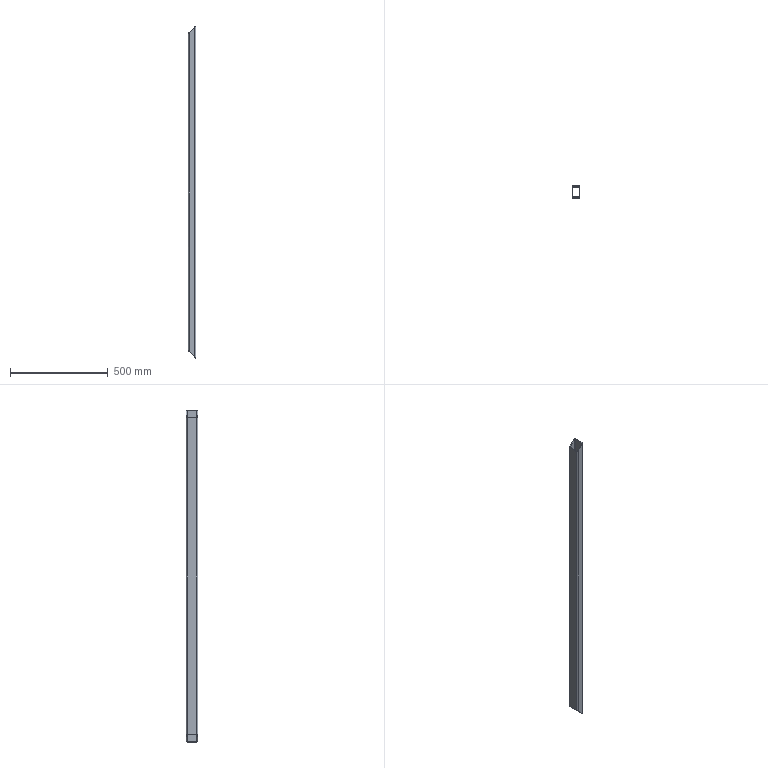Part | STEP file | Profile 40601700 | 1 solid | 18 faces | box 40 x 60 x 1700 mm | volume 950632 mm3 | plane 10 | cylinder 8 | commonest cylinder face diameters 6.4 x4 12.8 x4
STEP:
#1=CARTESIAN_POINT('',(40.,6.4,1100.));
#2=VERTEX_POINT('',#1);
#3=CARTESIAN_POINT('',(40.,53.6,1100.));
#4=VERTEX_POINT('',#3);
#5=CARTESIAN_POINT('',(40.,53.6,1100.));
#6=DIRECTION('',(0.,1.,0.));
#7=VECTOR('',#6,1000.);
#8=LINE('',#5,#7);
#9=EDGE_CURVE('',#2,#4,#8,.T.);
#10=ORIENTED_EDGE('',*,*,#9,.F.);
#11=CARTESIAN_POINT('',(40.,6.4,-600.));
#12=VERTEX_POINT('',#11);
#13=CARTESIAN_POINT('',(40.,6.4,600.));
#14=DIRECTION('',(0.,0.,1.));
#15=VECTOR('',#14,1000.);
#16=LINE('',#13,#15);
#17=EDGE_CURVE('',#12,#2,#16,.T.);
#18=ORIENTED_EDGE('',*,*,#17,.F.);
#19=CARTESIAN_POINT('',(40.,53.6,-600.));
#20=VERTEX_POINT('',#19);
#21=CARTESIAN_POINT('',(40.,53.6,-600.));
#22=DIRECTION('',(0.,-1.,0.));
#23=VECTOR('',#22,1000.);
#24=LINE('',#21,#23);
#25=EDGE_CURVE('',#20,#12,#24,.T.);
#26=ORIENTED_EDGE('',*,*,#25,.F.);
#27=CARTESIAN_POINT('',(40.,53.6,600.));
#28=DIRECTION('',(0.,0.,-1.));
#29=VECTOR('',#28,1000.);
#30=LINE('',#27,#29);
#31=EDGE_CURVE('',#4,#20,#30,.T.);
#32=ORIENTED_EDGE('',*,*,#31,.F.);
#33=EDGE_LOOP('',(#10,#18,#26,#32));
#34=FACE_OUTER_BOUND('',#33,.T.);
#35=CARTESIAN_POINT('',(40.,53.6,600.));
#36=DIRECTION('',(-1.,0.,0.));
#37=DIRECTION('',(0.,0.,1.));
#38=AXIS2_PLACEMENT_3D('',#35,#36,#37);
#39=PLANE('',#38);
#40=ADVANCED_FACE('',(#34),#39,.F.);
#41=CARTESIAN_POINT('',(33.6,60.,-593.6));
#42=VERTEX_POINT('',#41);
#43=CARTESIAN_POINT('',(40.,53.6,-600.));
#44=CARTESIAN_POINT('',(40.,57.349,-600.));
#45=CARTESIAN_POINT('',(37.349,60.,-597.349));
#46=CARTESIAN_POINT('',(33.6,60.,-593.6));
#47=(BOUNDED_CURVE()B_SPLINE_CURVE(3,(#43,#44,#45,#46),.UNSPECIFIED.,.F.,.F.)B_SPLINE_CURVE_WITH_KNOTS((4,4),(0.,1.571),.UNSPECIFIED.)CURVE()GEOMETRIC_REPRESENTATION_ITEM()RATIONAL_B_SPLINE_CURVE((1.,0.8047,0.8047,1.))REPRESENTATION_ITEM(''));
#48=EDGE_CURVE('',#20,#42,#47,.T.);
#49=ORIENTED_EDGE('',*,*,#48,.T.);
#50=CARTESIAN_POINT('',(33.6,60.,1093.6));
#51=VERTEX_POINT('',#50);
#52=CARTESIAN_POINT('',(33.6,60.,600.));
#53=DIRECTION('',(0.,0.,1.));
#54=VECTOR('',#53,1000.);
#55=LINE('',#52,#54);
#56=EDGE_CURVE('',#42,#51,#55,.T.);
#57=ORIENTED_EDGE('',*,*,#56,.T.);
#58=CARTESIAN_POINT('',(33.6,60.,1093.6));
#59=CARTESIAN_POINT('',(37.349,60.,1097.349));
#60=CARTESIAN_POINT('',(40.,57.349,1100.));
#61=CARTESIAN_POINT('',(40.,53.6,1100.));
#62=(BOUNDED_CURVE()B_SPLINE_CURVE(3,(#58,#59,#60,#61),.UNSPECIFIED.,.F.,.F.)B_SPLINE_CURVE_WITH_KNOTS((4,4),(1.571,3.142),.UNSPECIFIED.)CURVE()GEOMETRIC_REPRESENTATION_ITEM()RATIONAL_B_SPLINE_CURVE((1.,0.8047,0.8047,1.))REPRESENTATION_ITEM(''));
#63=EDGE_CURVE('',#51,#4,#62,.T.);
#64=ORIENTED_EDGE('',*,*,#63,.T.);
#65=ORIENTED_EDGE('',*,*,#31,.T.);
#66=EDGE_LOOP('',(#49,#57,#64,#65));
#67=FACE_OUTER_BOUND('',#66,.T.);
#68=CARTESIAN_POINT('',(33.6,53.6,600.));
#69=DIRECTION('',(0.,0.,-1.));
#70=DIRECTION('',(-1.,0.,0.));
#71=AXIS2_PLACEMENT_3D('',#68,#69,#70);
#72=CYLINDRICAL_SURFACE('',#71,6.4);
#73=ADVANCED_FACE('',(#67),#72,.T.);
#74=CARTESIAN_POINT('',(36.8,53.6,1096.8));
#75=VERTEX_POINT('',#74);
#76=CARTESIAN_POINT('',(33.6,56.8,1093.6));
#77=VERTEX_POINT('',#76);
#78=CARTESIAN_POINT('',(36.8,53.6,1096.8));
#79=CARTESIAN_POINT('',(36.8,55.475,1096.8));
#80=CARTESIAN_POINT('',(35.475,56.8,1095.475));
#81=CARTESIAN_POINT('',(33.6,56.8,1093.6));
#82=(BOUNDED_CURVE()B_SPLINE_CURVE(3,(#78,#79,#80,#81),.UNSPECIFIED.,.F.,.F.)B_SPLINE_CURVE_WITH_KNOTS((4,4),(3.142,4.712),.UNSPECIFIED.)CURVE()GEOMETRIC_REPRESENTATION_ITEM()RATIONAL_B_SPLINE_CURVE((1.,0.8047,0.8047,1.))REPRESENTATION_ITEM(''));
#83=EDGE_CURVE('',#75,#77,#82,.T.);
#84=ORIENTED_EDGE('',*,*,#83,.F.);
#85=CARTESIAN_POINT('',(36.8,6.4,1096.8));
#86=VERTEX_POINT('',#85);
#87=CARTESIAN_POINT('',(36.8,-440.,1096.8));
#88=DIRECTION('',(0.,1.,0.));
#89=VECTOR('',#88,1000.);
#90=LINE('',#87,#89);
#91=EDGE_CURVE('',#86,#75,#90,.T.);
#92=ORIENTED_EDGE('',*,*,#91,.F.);
#93=CARTESIAN_POINT('',(33.6,3.2,1093.6));
#94=VERTEX_POINT('',#93);
#95=CARTESIAN_POINT('',(33.6,3.2,1093.6));
#96=CARTESIAN_POINT('',(35.475,3.2,1095.475));
#97=CARTESIAN_POINT('',(36.8,4.525,1096.8));
#98=CARTESIAN_POINT('',(36.8,6.4,1096.8));
#99=(BOUNDED_CURVE()B_SPLINE_CURVE(3,(#95,#96,#97,#98),.UNSPECIFIED.,.F.,.T.)B_SPLINE_CURVE_WITH_KNOTS((4,4),(1.571,3.142),.UNSPECIFIED.)CURVE()GEOMETRIC_REPRESENTATION_ITEM()RATIONAL_B_SPLINE_CURVE((1.,0.8047,0.8047,1.))REPRESENTATION_ITEM(''));
#100=EDGE_CURVE('',#94,#86,#99,.T.);
#101=ORIENTED_EDGE('',*,*,#100,.F.);
#102=CARTESIAN_POINT('',(6.4,3.2,1066.4));
#103=VERTEX_POINT('',#102);
#104=CARTESIAN_POINT('',(0.,3.2,1060.));
#105=DIRECTION('',(0.7071,0.,0.7071));
#106=VECTOR('',#105,1000.);
#107=LINE('',#104,#106);
#108=EDGE_CURVE('',#103,#94,#107,.T.);
#109=ORIENTED_EDGE('',*,*,#108,.F.);
#110=CARTESIAN_POINT('',(3.2,6.4,1063.2));
#111=VERTEX_POINT('',#110);
#112=CARTESIAN_POINT('',(3.2,6.4,1063.2));
#113=CARTESIAN_POINT('',(3.2,4.525,1063.2));
#114=CARTESIAN_POINT('',(4.525,3.2,1064.525));
#115=CARTESIAN_POINT('',(6.4,3.2,1066.4));
#116=(BOUNDED_CURVE()B_SPLINE_CURVE(3,(#112,#113,#114,#115),.UNSPECIFIED.,.F.,.F.)B_SPLINE_CURVE_WITH_KNOTS((4,4),(0.,1.571),.UNSPECIFIED.)CURVE()GEOMETRIC_REPRESENTATION_ITEM()RATIONAL_B_SPLINE_CURVE((1.,0.8047,0.8047,1.))REPRESENTATION_ITEM(''));
#117=EDGE_CURVE('',#111,#103,#116,.T.);
#118=ORIENTED_EDGE('',*,*,#117,.F.);
#119=CARTESIAN_POINT('',(3.2,53.6,1063.2));
#120=VERTEX_POINT('',#119);
#121=CARTESIAN_POINT('',(3.2,-440.,1063.2));
#122=DIRECTION('',(0.,-1.,0.));
#123=VECTOR('',#122,1000.);
#124=LINE('',#121,#123);
#125=EDGE_CURVE('',#120,#111,#124,.T.);
#126=ORIENTED_EDGE('',*,*,#125,.F.);
#127=CARTESIAN_POINT('',(6.4,56.8,1066.4));
#128=VERTEX_POINT('',#127);
#129=CARTESIAN_POINT('',(6.4,56.8,1066.4));
#130=CARTESIAN_POINT('',(4.525,56.8,1064.525));
#131=CARTESIAN_POINT('',(3.2,55.475,1063.2));
#132=CARTESIAN_POINT('',(3.2,53.6,1063.2));
#133=(BOUNDED_CURVE()B_SPLINE_CURVE(3,(#129,#130,#131,#132),.UNSPECIFIED.,.F.,.F.)B_SPLINE_CURVE_WITH_KNOTS((4,4),(4.712,6.283),.UNSPECIFIED.)CURVE()GEOMETRIC_REPRESENTATION_ITEM()RATIONAL_B_SPLINE_CURVE((1.,0.8047,0.8047,1.))REPRESENTATION_ITEM(''));
#134=EDGE_CURVE('',#128,#120,#133,.T.);
#135=ORIENTED_EDGE('',*,*,#134,.F.);
#136=CARTESIAN_POINT('',(0.,56.8,1060.));
#137=DIRECTION('',(-0.7071,0.,-0.7071));
#138=VECTOR('',#137,1000.);
#139=LINE('',#136,#138);
#140=EDGE_CURVE('',#77,#128,#139,.T.);
#141=ORIENTED_EDGE('',*,*,#140,.F.);
#142=EDGE_LOOP('',(#84,#92,#101,#109,#118,#126,#135,#141));
#143=FACE_BOUND('',#142,.T.);
#144=CARTESIAN_POINT('',(6.4,60.,1066.4));
#145=VERTEX_POINT('',#144);
#146=CARTESIAN_POINT('',(0.,60.,1060.));
#147=DIRECTION('',(0.7071,0.,0.7071));
#148=VECTOR('',#147,1000.);
#149=LINE('',#146,#148);
#150=EDGE_CURVE('',#145,#51,#149,.T.);
#151=ORIENTED_EDGE('',*,*,#150,.F.);
#152=CARTESIAN_POINT('',(0.,53.6,1060.));
#153=VERTEX_POINT('',#152);
#154=CARTESIAN_POINT('',(0.,53.6,1060.));
#155=CARTESIAN_POINT('',(0.,57.349,1060.));
#156=CARTESIAN_POINT('',(2.651,60.,1062.651));
#157=CARTESIAN_POINT('',(6.4,60.,1066.4));
#158=(BOUNDED_CURVE()B_SPLINE_CURVE(3,(#154,#155,#156,#157),.UNSPECIFIED.,.F.,.T.)B_SPLINE_CURVE_WITH_KNOTS((4,4),(0.,1.571),.UNSPECIFIED.)CURVE()GEOMETRIC_REPRESENTATION_ITEM()RATIONAL_B_SPLINE_CURVE((1.,0.8047,0.8047,1.))REPRESENTATION_ITEM(''));
#159=EDGE_CURVE('',#153,#145,#158,.T.);
#160=ORIENTED_EDGE('',*,*,#159,.F.);
#161=CARTESIAN_POINT('',(0.,6.4,1060.));
#162=VERTEX_POINT('',#161);
#163=CARTESIAN_POINT('',(0.,-440.,1060.));
#164=DIRECTION('',(0.,1.,0.));
#165=VECTOR('',#164,1000.);
#166=LINE('',#163,#165);
#167=EDGE_CURVE('',#162,#153,#166,.T.);
#168=ORIENTED_EDGE('',*,*,#167,.F.);
#169=CARTESIAN_POINT('',(6.4,0.,1066.4));
#170=VERTEX_POINT('',#169);
#171=CARTESIAN_POINT('',(6.4,0.,1066.4));
#172=CARTESIAN_POINT('',(2.651,0.,1062.651));
#173=CARTESIAN_POINT('',(0.,2.651,1060.));
#174=CARTESIAN_POINT('',(0.,6.4,1060.));
#175=(BOUNDED_CURVE()B_SPLINE_CURVE(3,(#171,#172,#173,#174),.UNSPECIFIED.,.F.,.F.)B_SPLINE_CURVE_WITH_KNOTS((4,4),(4.712,6.283),.UNSPECIFIED.)CURVE()GEOMETRIC_REPRESENTATION_ITEM()RATIONAL_B_SPLINE_CURVE((1.,0.8047,0.8047,1.))REPRESENTATION_ITEM(''));
#176=EDGE_CURVE('',#170,#162,#175,.T.);
#177=ORIENTED_EDGE('',*,*,#176,.F.);
#178=CARTESIAN_POINT('',(33.6,0.,1093.6));
#179=VERTEX_POINT('',#178);
#180=CARTESIAN_POINT('',(0.,0.,1060.));
#181=DIRECTION('',(-0.7071,0.,-0.7071));
#182=VECTOR('',#181,1000.);
#183=LINE('',#180,#182);
#184=EDGE_CURVE('',#179,#170,#183,.T.);
#185=ORIENTED_EDGE('',*,*,#184,.F.);
#186=CARTESIAN_POINT('',(40.,6.4,1100.));
#187=CARTESIAN_POINT('',(40.,2.651,1100.));
#188=CARTESIAN_POINT('',(37.349,0.,1097.349));
#189=CARTESIAN_POINT('',(33.6,0.,1093.6));
#190=(BOUNDED_CURVE()B_SPLINE_CURVE(3,(#186,#187,#188,#189),.UNSPECIFIED.,.F.,.F.)B_SPLINE_CURVE_WITH_KNOTS((4,4),(3.142,4.712),.UNSPECIFIED.)CURVE()GEOMETRIC_REPRESENTATION_ITEM()RATIONAL_B_SPLINE_CURVE((1.,0.8047,0.8047,1.))REPRESENTATION_ITEM(''));
#191=EDGE_CURVE('',#2,#179,#190,.T.);
#192=ORIENTED_EDGE('',*,*,#191,.F.);
#193=ORIENTED_EDGE('',*,*,#9,.T.);
#194=ORIENTED_EDGE('',*,*,#63,.F.);
#195=EDGE_LOOP('',(#151,#160,#168,#177,#185,#192,#193,#194));
#196=FACE_OUTER_BOUND('',#195,.T.);
#197=CARTESIAN_POINT('',(0.,-440.,1060.));
#198=DIRECTION('',(0.7071,0.,-0.7071));
#199=DIRECTION('',(-0.7071,0.,-0.7071));
#200=AXIS2_PLACEMENT_3D('',#197,#198,#199);
#201=PLANE('',#200);
#202=ADVANCED_FACE('',(#143,#196),#201,.F.);
#203=CARTESIAN_POINT('',(33.6,0.,-593.6));
#204=VERTEX_POINT('',#203);
#205=CARTESIAN_POINT('',(33.6,0.,-593.6));
#206=CARTESIAN_POINT('',(37.349,0.,-597.349));
#207=CARTESIAN_POINT('',(40.,2.651,-600.));
#208=CARTESIAN_POINT('',(40.,6.4,-600.));
#209=(BOUNDED_CURVE()B_SPLINE_CURVE(3,(#205,#206,#207,#208),.UNSPECIFIED.,.F.,.F.)B_SPLINE_CURVE_WITH_KNOTS((4,4),(4.712,6.283),.UNSPECIFIED.)CURVE()GEOMETRIC_REPRESENTATION_ITEM()RATIONAL_B_SPLINE_CURVE((1.,0.8047,0.8047,1.))REPRESENTATION_ITEM(''));
#210=EDGE_CURVE('',#204,#12,#209,.T.);
#211=ORIENTED_EDGE('',*,*,#210,.T.);
#212=ORIENTED_EDGE('',*,*,#17,.T.);
#213=ORIENTED_EDGE('',*,*,#191,.T.);
#214=CARTESIAN_POINT('',(33.6,0.,600.));
#215=DIRECTION('',(0.,0.,-1.));
#216=VECTOR('',#215,1000.);
#217=LINE('',#214,#216);
#218=EDGE_CURVE('',#179,#204,#217,.T.);
#219=ORIENTED_EDGE('',*,*,#218,.T.);
#220=EDGE_LOOP('',(#211,#212,#213,#219));
#221=FACE_OUTER_BOUND('',#220,.T.);
#222=CARTESIAN_POINT('',(33.6,6.4,600.));
#223=DIRECTION('',(0.,0.,-1.));
#224=DIRECTION('',(-1.,0.,0.));
#225=AXIS2_PLACEMENT_3D('',#222,#223,#224);
#226=CYLINDRICAL_SURFACE('',#225,6.4);
#227=ADVANCED_FACE('',(#221),#226,.T.);
#228=CARTESIAN_POINT('',(3.2,53.6,-563.2));
#229=VERTEX_POINT('',#228);
#230=CARTESIAN_POINT('',(6.4,56.8,-566.4));
#231=VERTEX_POINT('',#230);
#232=CARTESIAN_POINT('',(3.2,53.6,-563.2));
#233=CARTESIAN_POINT('',(3.2,55.475,-563.2));
#234=CARTESIAN_POINT('',(4.525,56.8,-564.525));
#235=CARTESIAN_POINT('',(6.4,56.8,-566.4));
#236=(BOUNDED_CURVE()B_SPLINE_CURVE(3,(#232,#233,#234,#235),.UNSPECIFIED.,.F.,.T.)B_SPLINE_CURVE_WITH_KNOTS((4,4),(3.142,4.712),.UNSPECIFIED.)CURVE()GEOMETRIC_REPRESENTATION_ITEM()RATIONAL_B_SPLINE_CURVE((1.,0.8047,0.8047,1.))REPRESENTATION_ITEM(''));
#237=EDGE_CURVE('',#229,#231,#236,.T.);
#238=ORIENTED_EDGE('',*,*,#237,.F.);
#239=CARTESIAN_POINT('',(3.2,6.4,-563.2));
#240=VERTEX_POINT('',#239);
#241=CARTESIAN_POINT('',(3.2,-440.,-563.2));
#242=DIRECTION('',(0.,1.,0.));
#243=VECTOR('',#242,1000.);
#244=LINE('',#241,#243);
#245=EDGE_CURVE('',#240,#229,#244,.T.);
#246=ORIENTED_EDGE('',*,*,#245,.F.);
#247=CARTESIAN_POINT('',(6.4,3.2,-566.4));
#248=VERTEX_POINT('',#247);
#249=CARTESIAN_POINT('',(6.4,3.2,-566.4));
#250=CARTESIAN_POINT('',(4.525,3.2,-564.525));
#251=CARTESIAN_POINT('',(3.2,4.525,-563.2));
#252=CARTESIAN_POINT('',(3.2,6.4,-563.2));
#253=(BOUNDED_CURVE()B_SPLINE_CURVE(3,(#249,#250,#251,#252),.UNSPECIFIED.,.F.,.F.)B_SPLINE_CURVE_WITH_KNOTS((4,4),(1.571,3.142),.UNSPECIFIED.)CURVE()GEOMETRIC_REPRESENTATION_ITEM()RATIONAL_B_SPLINE_CURVE((1.,0.8047,0.8047,1.))REPRESENTATION_ITEM(''));
#254=EDGE_CURVE('',#248,#240,#253,.T.);
#255=ORIENTED_EDGE('',*,*,#254,.F.);
#256=CARTESIAN_POINT('',(33.6,3.2,-593.6));
#257=VERTEX_POINT('',#256);
#258=CARTESIAN_POINT('',(40.,3.2,-600.));
#259=DIRECTION('',(-0.7071,0.,0.7071));
#260=VECTOR('',#259,1000.);
#261=LINE('',#258,#260);
#262=EDGE_CURVE('',#257,#248,#261,.T.);
#263=ORIENTED_EDGE('',*,*,#262,.F.);
#264=CARTESIAN_POINT('',(36.8,6.4,-596.8));
#265=VERTEX_POINT('',#264);
#266=CARTESIAN_POINT('',(36.8,6.4,-596.8));
#267=CARTESIAN_POINT('',(36.8,4.525,-596.8));
#268=CARTESIAN_POINT('',(35.475,3.2,-595.475));
#269=CARTESIAN_POINT('',(33.6,3.2,-593.6));
#270=(BOUNDED_CURVE()B_SPLINE_CURVE(3,(#266,#267,#268,#269),.UNSPECIFIED.,.F.,.F.)B_SPLINE_CURVE_WITH_KNOTS((4,4),(0.,1.571),.UNSPECIFIED.)CURVE()GEOMETRIC_REPRESENTATION_ITEM()RATIONAL_B_SPLINE_CURVE((1.,0.8047,0.8047,1.))REPRESENTATION_ITEM(''));
#271=EDGE_CURVE('',#265,#257,#270,.T.);
#272=ORIENTED_EDGE('',*,*,#271,.F.);
#273=CARTESIAN_POINT('',(36.8,53.6,-596.8));
#274=VERTEX_POINT('',#273);
#275=CARTESIAN_POINT('',(36.8,-440.,-596.8));
#276=DIRECTION('',(0.,-1.,0.));
#277=VECTOR('',#276,1000.);
#278=LINE('',#275,#277);
#279=EDGE_CURVE('',#274,#265,#278,.T.);
#280=ORIENTED_EDGE('',*,*,#279,.F.);
#281=CARTESIAN_POINT('',(33.6,56.8,-593.6));
#282=VERTEX_POINT('',#281);
#283=CARTESIAN_POINT('',(33.6,56.8,-593.6));
#284=CARTESIAN_POINT('',(35.475,56.8,-595.475));
#285=CARTESIAN_POINT('',(36.8,55.475,-596.8));
#286=CARTESIAN_POINT('',(36.8,53.6,-596.8));
#287=(BOUNDED_CURVE()B_SPLINE_CURVE(3,(#283,#284,#285,#286),.UNSPECIFIED.,.F.,.F.)B_SPLINE_CURVE_WITH_KNOTS((4,4),(4.712,6.283),.UNSPECIFIED.)CURVE()GEOMETRIC_REPRESENTATION_ITEM()RATIONAL_B_SPLINE_CURVE((1.,0.8047,0.8047,1.))REPRESENTATION_ITEM(''));
#288=EDGE_CURVE('',#282,#274,#287,.T.);
#289=ORIENTED_EDGE('',*,*,#288,.F.);
#290=CARTESIAN_POINT('',(40.,56.8,-600.));
#291=DIRECTION('',(0.7071,0.,-0.7071));
#292=VECTOR('',#291,1000.);
#293=LINE('',#290,#292);
#294=EDGE_CURVE('',#231,#282,#293,.T.);
#295=ORIENTED_EDGE('',*,*,#294,.F.);
#296=EDGE_LOOP('',(#238,#246,#255,#263,#272,#280,#289,#295));
#297=FACE_BOUND('',#296,.T.);
#298=ORIENTED_EDGE('',*,*,#25,.T.);
#299=ORIENTED_EDGE('',*,*,#210,.F.);
#300=CARTESIAN_POINT('',(6.4,0.,-566.4));
#301=VERTEX_POINT('',#300);
#302=CARTESIAN_POINT('',(40.,0.,-600.));
#303=DIRECTION('',(0.7071,0.,-0.7071));
#304=VECTOR('',#303,1000.);
#305=LINE('',#302,#304);
#306=EDGE_CURVE('',#301,#204,#305,.T.);
#307=ORIENTED_EDGE('',*,*,#306,.F.);
#308=CARTESIAN_POINT('',(0.,6.4,-560.));
#309=VERTEX_POINT('',#308);
#310=CARTESIAN_POINT('',(0.,6.4,-560.));
#311=CARTESIAN_POINT('',(0.,2.651,-560.));
#312=CARTESIAN_POINT('',(2.651,0.,-562.651));
#313=CARTESIAN_POINT('',(6.4,0.,-566.4));
#314=(BOUNDED_CURVE()B_SPLINE_CURVE(3,(#310,#311,#312,#313),.UNSPECIFIED.,.F.,.F.)B_SPLINE_CURVE_WITH_KNOTS((4,4),(3.142,4.712),.UNSPECIFIED.)CURVE()GEOMETRIC_REPRESENTATION_ITEM()RATIONAL_B_SPLINE_CURVE((1.,0.8047,0.8047,1.))REPRESENTATION_ITEM(''));
#315=EDGE_CURVE('',#309,#301,#314,.T.);
#316=ORIENTED_EDGE('',*,*,#315,.F.);
#317=CARTESIAN_POINT('',(0.,53.6,-560.));
#318=VERTEX_POINT('',#317);
#319=CARTESIAN_POINT('',(0.,-440.,-560.));
#320=DIRECTION('',(0.,-1.,0.));
#321=VECTOR('',#320,1000.);
#322=LINE('',#319,#321);
#323=EDGE_CURVE('',#318,#309,#322,.T.);
#324=ORIENTED_EDGE('',*,*,#323,.F.);
#325=CARTESIAN_POINT('',(6.4,60.,-566.4));
#326=VERTEX_POINT('',#325);
#327=CARTESIAN_POINT('',(6.4,60.,-566.4));
#328=CARTESIAN_POINT('',(2.651,60.,-562.651));
#329=CARTESIAN_POINT('',(0.,57.349,-560.));
#330=CARTESIAN_POINT('',(0.,53.6,-560.));
#331=(BOUNDED_CURVE()B_SPLINE_CURVE(3,(#327,#328,#329,#330),.UNSPECIFIED.,.F.,.F.)B_SPLINE_CURVE_WITH_KNOTS((4,4),(1.571,3.142),.UNSPECIFIED.)CURVE()GEOMETRIC_REPRESENTATION_ITEM()RATIONAL_B_SPLINE_CURVE((1.,0.8047,0.8047,1.))REPRESENTATION_ITEM(''));
#332=EDGE_CURVE('',#326,#318,#331,.T.);
#333=ORIENTED_EDGE('',*,*,#332,.F.);
#334=CARTESIAN_POINT('',(40.,60.,-600.));
#335=DIRECTION('',(-0.7071,0.,0.7071));
#336=VECTOR('',#335,1000.);
#337=LINE('',#334,#336);
#338=EDGE_CURVE('',#42,#326,#337,.T.);
#339=ORIENTED_EDGE('',*,*,#338,.F.);
#340=ORIENTED_EDGE('',*,*,#48,.F.);
#341=EDGE_LOOP('',(#298,#299,#307,#316,#324,#333,#339,#340));
#342=FACE_OUTER_BOUND('',#341,.T.);
#343=CARTESIAN_POINT('',(40.,-440.,-600.));
#344=DIRECTION('',(0.7071,0.,0.7071));
#345=DIRECTION('',(0.7071,0.,-0.7071));
#346=AXIS2_PLACEMENT_3D('',#343,#344,#345);
#347=PLANE('',#346);
#348=ADVANCED_FACE('',(#297,#342),#347,.F.);
#349=ORIENTED_EDGE('',*,*,#150,.T.);
#350=ORIENTED_EDGE('',*,*,#56,.F.);
#351=ORIENTED_EDGE('',*,*,#338,.T.);
#352=CARTESIAN_POINT('',(6.4,60.,600.));
#353=DIRECTION('',(0.,0.,-1.));
#354=VECTOR('',#353,1000.);
#355=LINE('',#352,#354);
#356=EDGE_CURVE('',#145,#326,#355,.T.);
#357=ORIENTED_EDGE('',*,*,#356,.F.);
#358=EDGE_LOOP('',(#349,#350,#351,#357));
#359=FACE_OUTER_BOUND('',#358,.T.);
#360=CARTESIAN_POINT('',(33.6,60.,600.));
#361=DIRECTION('',(0.,-1.,0.));
#362=DIRECTION('',(0.,0.,-1.));
#363=AXIS2_PLACEMENT_3D('',#360,#361,#362);
#364=PLANE('',#363);
#365=ADVANCED_FACE('',(#359),#364,.F.);
#366=ORIENTED_EDGE('',*,*,#294,.T.);
#367=CARTESIAN_POINT('',(33.6,56.8,600.));
#368=DIRECTION('',(0.,0.,1.));
#369=VECTOR('',#368,1000.);
#370=LINE('',#367,#369);
#371=EDGE_CURVE('',#282,#77,#370,.T.);
#372=ORIENTED_EDGE('',*,*,#371,.T.);
#373=ORIENTED_EDGE('',*,*,#140,.T.);
#374=CARTESIAN_POINT('',(6.4,56.8,600.));
#375=DIRECTION('',(0.,0.,-1.));
#376=VECTOR('',#375,1000.);
#377=LINE('',#374,#376);
#378=EDGE_CURVE('',#128,#231,#377,.T.);
#379=ORIENTED_EDGE('',*,*,#378,.T.);
#380=EDGE_LOOP('',(#366,#372,#373,#379));
#381=FACE_OUTER_BOUND('',#380,.T.);
#382=CARTESIAN_POINT('',(33.6,56.8,600.));
#383=DIRECTION('',(0.,-1.,0.));
#384=DIRECTION('',(0.,0.,-1.));
#385=AXIS2_PLACEMENT_3D('',#382,#383,#384);
#386=PLANE('',#385);
#387=ADVANCED_FACE('',(#381),#386,.T.);
#388=ORIENTED_EDGE('',*,*,#83,.T.);
#389=ORIENTED_EDGE('',*,*,#371,.F.);
#390=ORIENTED_EDGE('',*,*,#288,.T.);
#391=CARTESIAN_POINT('',(36.8,53.6,600.));
#392=DIRECTION('',(0.,0.,-1.));
#393=VECTOR('',#392,1000.);
#394=LINE('',#391,#393);
#395=EDGE_CURVE('',#75,#274,#394,.T.);
#396=ORIENTED_EDGE('',*,*,#395,.F.);
#397=EDGE_LOOP('',(#388,#389,#390,#396));
#398=FACE_OUTER_BOUND('',#397,.T.);
#399=CARTESIAN_POINT('',(33.6,53.6,600.));
#400=DIRECTION('',(0.,0.,-1.));
#401=DIRECTION('',(-1.,0.,0.));
#402=AXIS2_PLACEMENT_3D('',#399,#400,#401);
#403=CYLINDRICAL_SURFACE('',#402,3.2);
#404=ADVANCED_FACE('',(#398),#403,.F.);
#405=ORIENTED_EDGE('',*,*,#279,.T.);
#406=CARTESIAN_POINT('',(36.8,6.4,600.));
#407=DIRECTION('',(0.,0.,1.));
#408=VECTOR('',#407,1000.);
#409=LINE('',#406,#408);
#410=EDGE_CURVE('',#265,#86,#409,.T.);
#411=ORIENTED_EDGE('',*,*,#410,.T.);
#412=ORIENTED_EDGE('',*,*,#91,.T.);
#413=ORIENTED_EDGE('',*,*,#395,.T.);
#414=EDGE_LOOP('',(#405,#411,#412,#413));
#415=FACE_OUTER_BOUND('',#414,.T.);
#416=CARTESIAN_POINT('',(36.8,53.6,600.));
#417=DIRECTION('',(-1.,0.,0.));
#418=DIRECTION('',(0.,0.,1.));
#419=AXIS2_PLACEMENT_3D('',#416,#417,#418);
#420=PLANE('',#419);
#421=ADVANCED_FACE('',(#415),#420,.T.);
#422=ORIENTED_EDGE('',*,*,#100,.T.);
#423=ORIENTED_EDGE('',*,*,#410,.F.);
#424=ORIENTED_EDGE('',*,*,#271,.T.);
#425=CARTESIAN_POINT('',(33.6,3.2,600.));
#426=DIRECTION('',(0.,0.,-1.));
#427=VECTOR('',#426,1000.);
#428=LINE('',#425,#427);
#429=EDGE_CURVE('',#94,#257,#428,.T.);
#430=ORIENTED_EDGE('',*,*,#429,.F.);
#431=EDGE_LOOP('',(#422,#423,#424,#430));
#432=FACE_OUTER_BOUND('',#431,.T.);
#433=CARTESIAN_POINT('',(33.6,6.4,600.));
#434=DIRECTION('',(0.,0.,-1.));
#435=DIRECTION('',(-1.,0.,0.));
#436=AXIS2_PLACEMENT_3D('',#433,#434,#435);
#437=CYLINDRICAL_SURFACE('',#436,3.2);
#438=ADVANCED_FACE('',(#432),#437,.F.);
#439=ORIENTED_EDGE('',*,*,#262,.T.);
#440=CARTESIAN_POINT('',(6.4,3.2,600.));
#441=DIRECTION('',(0.,0.,1.));
#442=VECTOR('',#441,1000.);
#443=LINE('',#440,#442);
#444=EDGE_CURVE('',#248,#103,#443,.T.);
#445=ORIENTED_EDGE('',*,*,#444,.T.);
#446=ORIENTED_EDGE('',*,*,#108,.T.);
#447=ORIENTED_EDGE('',*,*,#429,.T.);
#448=EDGE_LOOP('',(#439,#445,#446,#447));
#449=FACE_OUTER_BOUND('',#448,.T.);
#450=CARTESIAN_POINT('',(6.4,3.2,600.));
#451=DIRECTION('',(0.,1.,0.));
#452=DIRECTION('',(-1.,0.,0.));
#453=AXIS2_PLACEMENT_3D('',#450,#451,#452);
#454=PLANE('',#453);
#455=ADVANCED_FACE('',(#449),#454,.T.);
#456=ORIENTED_EDGE('',*,*,#117,.T.);
#457=ORIENTED_EDGE('',*,*,#444,.F.);
#458=ORIENTED_EDGE('',*,*,#254,.T.);
#459=CARTESIAN_POINT('',(3.2,6.4,600.));
#460=DIRECTION('',(0.,0.,-1.));
#461=VECTOR('',#460,1000.);
#462=LINE('',#459,#461);
#463=EDGE_CURVE('',#111,#240,#462,.T.);
#464=ORIENTED_EDGE('',*,*,#463,.F.);
#465=EDGE_LOOP('',(#456,#457,#458,#464));
#466=FACE_OUTER_BOUND('',#465,.T.);
#467=CARTESIAN_POINT('',(6.4,6.4,600.));
#468=DIRECTION('',(0.,0.,-1.));
#469=DIRECTION('',(-1.,0.,0.));
#470=AXIS2_PLACEMENT_3D('',#467,#468,#469);
#471=CYLINDRICAL_SURFACE('',#470,3.2);
#472=ADVANCED_FACE('',(#466),#471,.F.);
#473=ORIENTED_EDGE('',*,*,#245,.T.);
#474=CARTESIAN_POINT('',(3.2,53.6,600.));
#475=DIRECTION('',(0.,0.,1.));
#476=VECTOR('',#475,1000.);
#477=LINE('',#474,#476);
#478=EDGE_CURVE('',#229,#120,#477,.T.);
#479=ORIENTED_EDGE('',*,*,#478,.T.);
#480=ORIENTED_EDGE('',*,*,#125,.T.);
#481=ORIENTED_EDGE('',*,*,#463,.T.);
#482=EDGE_LOOP('',(#473,#479,#480,#481));
#483=FACE_OUTER_BOUND('',#482,.T.);
#484=CARTESIAN_POINT('',(3.2,6.4,600.));
#485=DIRECTION('',(1.,0.,0.));
#486=DIRECTION('',(0.,1.,0.));
#487=AXIS2_PLACEMENT_3D('',#484,#485,#486);
#488=PLANE('',#487);
#489=ADVANCED_FACE('',(#483),#488,.T.);
#490=ORIENTED_EDGE('',*,*,#134,.T.);
#491=ORIENTED_EDGE('',*,*,#478,.F.);
#492=ORIENTED_EDGE('',*,*,#237,.T.);
#493=ORIENTED_EDGE('',*,*,#378,.F.);
#494=EDGE_LOOP('',(#490,#491,#492,#493));
#495=FACE_OUTER_BOUND('',#494,.T.);
#496=CARTESIAN_POINT('',(6.4,53.6,600.));
#497=DIRECTION('',(0.,0.,-1.));
#498=DIRECTION('',(-1.,0.,0.));
#499=AXIS2_PLACEMENT_3D('',#496,#497,#498);
#500=CYLINDRICAL_SURFACE('',#499,3.2);
#501=ADVANCED_FACE('',(#495),#500,.F.);
#502=ORIENTED_EDGE('',*,*,#332,.T.);
#503=CARTESIAN_POINT('',(0.,53.6,600.));
#504=DIRECTION('',(0.,0.,1.));
#505=VECTOR('',#504,1000.);
#506=LINE('',#503,#505);
#507=EDGE_CURVE('',#318,#153,#506,.T.);
#508=ORIENTED_EDGE('',*,*,#507,.T.);
#509=ORIENTED_EDGE('',*,*,#159,.T.);
#510=ORIENTED_EDGE('',*,*,#356,.T.);
#511=EDGE_LOOP('',(#502,#508,#509,#510));
#512=FACE_OUTER_BOUND('',#511,.T.);
#513=CARTESIAN_POINT('',(6.4,53.6,600.));
#514=DIRECTION('',(0.,0.,-1.));
#515=DIRECTION('',(-1.,0.,0.));
#516=AXIS2_PLACEMENT_3D('',#513,#514,#515);
#517=CYLINDRICAL_SURFACE('',#516,6.4);
#518=ADVANCED_FACE('',(#512),#517,.T.);
#519=ORIENTED_EDGE('',*,*,#167,.T.);
#520=ORIENTED_EDGE('',*,*,#507,.F.);
#521=ORIENTED_EDGE('',*,*,#323,.T.);
#522=CARTESIAN_POINT('',(0.,6.4,600.));
#523=DIRECTION('',(0.,0.,-1.));
#524=VECTOR('',#523,1000.);
#525=LINE('',#522,#524);
#526=EDGE_CURVE('',#162,#309,#525,.T.);
#527=ORIENTED_EDGE('',*,*,#526,.F.);
#528=EDGE_LOOP('',(#519,#520,#521,#527));
#529=FACE_OUTER_BOUND('',#528,.T.);
#530=CARTESIAN_POINT('',(0.,6.4,600.));
#531=DIRECTION('',(1.,0.,0.));
#532=DIRECTION('',(0.,1.,0.));
#533=AXIS2_PLACEMENT_3D('',#530,#531,#532);
#534=PLANE('',#533);
#535=ADVANCED_FACE('',(#529),#534,.F.);
#536=ORIENTED_EDGE('',*,*,#315,.T.);
#537=CARTESIAN_POINT('',(6.4,0.,600.));
#538=DIRECTION('',(0.,0.,1.));
#539=VECTOR('',#538,1000.);
#540=LINE('',#537,#539);
#541=EDGE_CURVE('',#301,#170,#540,.T.);
#542=ORIENTED_EDGE('',*,*,#541,.T.);
#543=ORIENTED_EDGE('',*,*,#176,.T.);
#544=ORIENTED_EDGE('',*,*,#526,.T.);
#545=EDGE_LOOP('',(#536,#542,#543,#544));
#546=FACE_OUTER_BOUND('',#545,.T.);
#547=CARTESIAN_POINT('',(6.4,6.4,600.));
#548=DIRECTION('',(0.,0.,-1.));
#549=DIRECTION('',(-1.,0.,0.));
#550=AXIS2_PLACEMENT_3D('',#547,#548,#549);
#551=CYLINDRICAL_SURFACE('',#550,6.4);
#552=ADVANCED_FACE('',(#546),#551,.T.);
#553=ORIENTED_EDGE('',*,*,#184,.T.);
#554=ORIENTED_EDGE('',*,*,#541,.F.);
#555=ORIENTED_EDGE('',*,*,#306,.T.);
#556=ORIENTED_EDGE('',*,*,#218,.F.);
#557=EDGE_LOOP('',(#553,#554,#555,#556));
#558=FACE_OUTER_BOUND('',#557,.T.);
#559=CARTESIAN_POINT('',(6.4,0.,600.));
#560=DIRECTION('',(0.,1.,0.));
#561=DIRECTION('',(-1.,0.,0.));
#562=AXIS2_PLACEMENT_3D('',#559,#560,#561);
#563=PLANE('',#562);
#564=ADVANCED_FACE('',(#558),#563,.F.);
#565=CLOSED_SHELL('',(#40,#73,#202,#227,#348,#365,#387,#404,#421,#438,#455,#472,#489,#501,#518,#535,#552,#564));
#566=MANIFOLD_SOLID_BREP('',#565);
#567=CARTESIAN_POINT('',(0.,0.,0.));
#568=DIRECTION('',(0.,0.,1.));
#569=DIRECTION('',(1.,0.,0.));
#570=AXIS2_PLACEMENT_3D('',#567,#568,#569);
#571=(LENGTH_UNIT()NAMED_UNIT(*)SI_UNIT(.MILLI.,.METRE.));
#572=UNCERTAINTY_MEASURE_WITH_UNIT(LENGTH_MEASURE(0.00001),#571,'','');
#573=(NAMED_UNIT(*)PLANE_ANGLE_UNIT()SI_UNIT($,.RADIAN.));
#574=(NAMED_UNIT(*)SI_UNIT($,.STERADIAN.)SOLID_ANGLE_UNIT());
#575=(GEOMETRIC_REPRESENTATION_CONTEXT(3)GLOBAL_UNCERTAINTY_ASSIGNED_CONTEXT((#572))GLOBAL_UNIT_ASSIGNED_CONTEXT((#571,#573,#574))REPRESENTATION_CONTEXT('',''));
#576=ADVANCED_BREP_SHAPE_REPRESENTATION('',(#566,#570),#575);